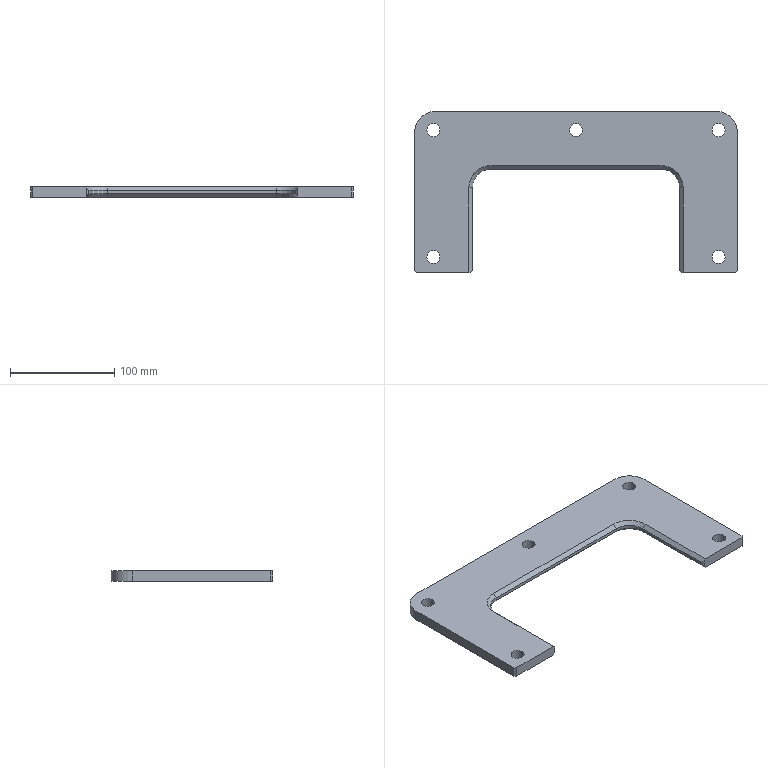Part | SolidWorks | features Chamfer 2, Extrusion 1, ICE 1 | 1 solid | 38 faces | box 310 x 155 x 10 mm | volume 271244 mm3 | plane 20 | cylinder 14 | cone 4 | commonest cylinder face diameters 12.5 x10 36 x2 40 x2
STEP:
#1=CARTESIAN_POINT('',(-143.25,15.,0.));
#2=VERTEX_POINT('',#1);
#3=CARTESIAN_POINT('',(-130.75,15.,0.));
#4=VERTEX_POINT('',#3);
#5=CARTESIAN_POINT('',(-137.,15.,0.));
#6=DIRECTION('',(0.,0.,1.));
#7=DIRECTION('',(1.,0.,0.));
#8=AXIS2_PLACEMENT_3D('',#5,#6,#7);
#9=CIRCLE('',#8,6.25);
#10=EDGE_CURVE('',#2,#4,#9,.T.);
#11=ORIENTED_EDGE('',*,*,#10,.F.);
#12=CARTESIAN_POINT('',(-143.25,15.,10.));
#13=VERTEX_POINT('',#12);
#14=CARTESIAN_POINT('',(-143.25,15.,0.));
#15=DIRECTION('',(0.,0.,1.));
#16=VECTOR('',#15,1000.);
#17=LINE('',#14,#16);
#18=EDGE_CURVE('',#2,#13,#17,.T.);
#19=ORIENTED_EDGE('',*,*,#18,.T.);
#20=CARTESIAN_POINT('',(-130.75,15.,10.));
#21=VERTEX_POINT('',#20);
#22=CARTESIAN_POINT('',(-137.,15.,10.));
#23=DIRECTION('',(0.,0.,1.));
#24=DIRECTION('',(1.,0.,0.));
#25=AXIS2_PLACEMENT_3D('',#22,#23,#24);
#26=CIRCLE('',#25,6.25);
#27=EDGE_CURVE('',#13,#21,#26,.T.);
#28=ORIENTED_EDGE('',*,*,#27,.T.);
#29=CARTESIAN_POINT('',(-130.75,15.,0.));
#30=DIRECTION('',(0.,0.,1.));
#31=VECTOR('',#30,1000.);
#32=LINE('',#29,#31);
#33=EDGE_CURVE('',#4,#21,#32,.T.);
#34=ORIENTED_EDGE('',*,*,#33,.F.);
#35=EDGE_LOOP('',(#11,#19,#28,#34));
#36=FACE_OUTER_BOUND('',#35,.T.);
#37=CARTESIAN_POINT('',(-137.,15.,0.));
#38=DIRECTION('',(0.,0.,1.));
#39=DIRECTION('',(1.,0.,0.));
#40=AXIS2_PLACEMENT_3D('',#37,#38,#39);
#41=CYLINDRICAL_SURFACE('',#40,6.25);
#42=ADVANCED_FACE('',(#36),#41,.F.);
#43=CARTESIAN_POINT('',(130.75,15.,0.));
#44=VERTEX_POINT('',#43);
#45=CARTESIAN_POINT('',(143.25,15.,0.));
#46=VERTEX_POINT('',#45);
#47=CARTESIAN_POINT('',(137.,15.,0.));
#48=DIRECTION('',(0.,0.,1.));
#49=DIRECTION('',(-1.,0.,0.));
#50=AXIS2_PLACEMENT_3D('',#47,#48,#49);
#51=CIRCLE('',#50,6.25);
#52=EDGE_CURVE('',#44,#46,#51,.T.);
#53=ORIENTED_EDGE('',*,*,#52,.F.);
#54=CARTESIAN_POINT('',(130.75,15.,10.));
#55=VERTEX_POINT('',#54);
#56=CARTESIAN_POINT('',(130.75,15.,0.));
#57=DIRECTION('',(0.,0.,1.));
#58=VECTOR('',#57,1000.);
#59=LINE('',#56,#58);
#60=EDGE_CURVE('',#44,#55,#59,.T.);
#61=ORIENTED_EDGE('',*,*,#60,.T.);
#62=CARTESIAN_POINT('',(143.25,15.,10.));
#63=VERTEX_POINT('',#62);
#64=CARTESIAN_POINT('',(137.,15.,10.));
#65=DIRECTION('',(0.,0.,1.));
#66=DIRECTION('',(-1.,0.,0.));
#67=AXIS2_PLACEMENT_3D('',#64,#65,#66);
#68=CIRCLE('',#67,6.25);
#69=EDGE_CURVE('',#55,#63,#68,.T.);
#70=ORIENTED_EDGE('',*,*,#69,.T.);
#71=CARTESIAN_POINT('',(143.25,15.,0.));
#72=DIRECTION('',(0.,0.,1.));
#73=VECTOR('',#72,1000.);
#74=LINE('',#71,#73);
#75=EDGE_CURVE('',#46,#63,#74,.T.);
#76=ORIENTED_EDGE('',*,*,#75,.F.);
#77=EDGE_LOOP('',(#53,#61,#70,#76));
#78=FACE_OUTER_BOUND('',#77,.T.);
#79=CARTESIAN_POINT('',(137.,15.,0.));
#80=DIRECTION('',(0.,0.,1.));
#81=DIRECTION('',(1.,0.,0.));
#82=AXIS2_PLACEMENT_3D('',#79,#80,#81);
#83=CYLINDRICAL_SURFACE('',#82,6.25);
#84=ADVANCED_FACE('',(#78),#83,.F.);
#85=CARTESIAN_POINT('',(-143.25,137.,0.));
#86=VERTEX_POINT('',#85);
#87=CARTESIAN_POINT('',(-130.75,137.,0.));
#88=VERTEX_POINT('',#87);
#89=CARTESIAN_POINT('',(-137.,137.,0.));
#90=DIRECTION('',(0.,0.,1.));
#91=DIRECTION('',(1.,0.,0.));
#92=AXIS2_PLACEMENT_3D('',#89,#90,#91);
#93=CIRCLE('',#92,6.25);
#94=EDGE_CURVE('',#86,#88,#93,.T.);
#95=ORIENTED_EDGE('',*,*,#94,.F.);
#96=CARTESIAN_POINT('',(-143.25,137.,10.));
#97=VERTEX_POINT('',#96);
#98=CARTESIAN_POINT('',(-143.25,137.,0.));
#99=DIRECTION('',(0.,0.,1.));
#100=VECTOR('',#99,1000.);
#101=LINE('',#98,#100);
#102=EDGE_CURVE('',#86,#97,#101,.T.);
#103=ORIENTED_EDGE('',*,*,#102,.T.);
#104=CARTESIAN_POINT('',(-130.75,137.,10.));
#105=VERTEX_POINT('',#104);
#106=CARTESIAN_POINT('',(-137.,137.,10.));
#107=DIRECTION('',(0.,0.,1.));
#108=DIRECTION('',(1.,0.,0.));
#109=AXIS2_PLACEMENT_3D('',#106,#107,#108);
#110=CIRCLE('',#109,6.25);
#111=EDGE_CURVE('',#97,#105,#110,.T.);
#112=ORIENTED_EDGE('',*,*,#111,.T.);
#113=CARTESIAN_POINT('',(-130.75,137.,0.));
#114=DIRECTION('',(0.,0.,1.));
#115=VECTOR('',#114,1000.);
#116=LINE('',#113,#115);
#117=EDGE_CURVE('',#88,#105,#116,.T.);
#118=ORIENTED_EDGE('',*,*,#117,.F.);
#119=EDGE_LOOP('',(#95,#103,#112,#118));
#120=FACE_OUTER_BOUND('',#119,.T.);
#121=CARTESIAN_POINT('',(-137.,137.,0.));
#122=DIRECTION('',(0.,0.,1.));
#123=DIRECTION('',(1.,0.,0.));
#124=AXIS2_PLACEMENT_3D('',#121,#122,#123);
#125=CYLINDRICAL_SURFACE('',#124,6.25);
#126=ADVANCED_FACE('',(#120),#125,.F.);
#127=CARTESIAN_POINT('',(130.75,137.,0.));
#128=VERTEX_POINT('',#127);
#129=CARTESIAN_POINT('',(143.25,137.,0.));
#130=VERTEX_POINT('',#129);
#131=CARTESIAN_POINT('',(137.,137.,0.));
#132=DIRECTION('',(0.,0.,1.));
#133=DIRECTION('',(1.,0.,0.));
#134=AXIS2_PLACEMENT_3D('',#131,#132,#133);
#135=CIRCLE('',#134,6.25);
#136=EDGE_CURVE('',#128,#130,#135,.T.);
#137=ORIENTED_EDGE('',*,*,#136,.F.);
#138=CARTESIAN_POINT('',(130.75,137.,10.));
#139=VERTEX_POINT('',#138);
#140=CARTESIAN_POINT('',(130.75,137.,0.));
#141=DIRECTION('',(0.,0.,1.));
#142=VECTOR('',#141,1000.);
#143=LINE('',#140,#142);
#144=EDGE_CURVE('',#128,#139,#143,.T.);
#145=ORIENTED_EDGE('',*,*,#144,.T.);
#146=CARTESIAN_POINT('',(143.25,137.,10.));
#147=VERTEX_POINT('',#146);
#148=CARTESIAN_POINT('',(137.,137.,10.));
#149=DIRECTION('',(0.,0.,1.));
#150=DIRECTION('',(1.,0.,0.));
#151=AXIS2_PLACEMENT_3D('',#148,#149,#150);
#152=CIRCLE('',#151,6.25);
#153=EDGE_CURVE('',#139,#147,#152,.T.);
#154=ORIENTED_EDGE('',*,*,#153,.T.);
#155=CARTESIAN_POINT('',(143.25,137.,0.));
#156=DIRECTION('',(0.,0.,1.));
#157=VECTOR('',#156,1000.);
#158=LINE('',#155,#157);
#159=EDGE_CURVE('',#130,#147,#158,.T.);
#160=ORIENTED_EDGE('',*,*,#159,.F.);
#161=EDGE_LOOP('',(#137,#145,#154,#160));
#162=FACE_OUTER_BOUND('',#161,.T.);
#163=CARTESIAN_POINT('',(137.,137.,0.));
#164=DIRECTION('',(0.,0.,1.));
#165=DIRECTION('',(1.,0.,0.));
#166=AXIS2_PLACEMENT_3D('',#163,#164,#165);
#167=CYLINDRICAL_SURFACE('',#166,6.25);
#168=ADVANCED_FACE('',(#162),#167,.F.);
#169=CARTESIAN_POINT('',(-6.25,137.,0.));
#170=VERTEX_POINT('',#169);
#171=CARTESIAN_POINT('',(6.25,137.,0.));
#172=VERTEX_POINT('',#171);
#173=CARTESIAN_POINT('',(0.,137.,0.));
#174=DIRECTION('',(0.,0.,1.));
#175=DIRECTION('',(1.,0.,0.));
#176=AXIS2_PLACEMENT_3D('',#173,#174,#175);
#177=CIRCLE('',#176,6.25);
#178=EDGE_CURVE('',#170,#172,#177,.T.);
#179=ORIENTED_EDGE('',*,*,#178,.F.);
#180=CARTESIAN_POINT('',(-6.25,137.,10.));
#181=VERTEX_POINT('',#180);
#182=CARTESIAN_POINT('',(-6.25,137.,0.));
#183=DIRECTION('',(0.,0.,1.));
#184=VECTOR('',#183,1000.);
#185=LINE('',#182,#184);
#186=EDGE_CURVE('',#170,#181,#185,.T.);
#187=ORIENTED_EDGE('',*,*,#186,.T.);
#188=CARTESIAN_POINT('',(6.25,137.,10.));
#189=VERTEX_POINT('',#188);
#190=CARTESIAN_POINT('',(0.,137.,10.));
#191=DIRECTION('',(0.,0.,1.));
#192=DIRECTION('',(1.,0.,0.));
#193=AXIS2_PLACEMENT_3D('',#190,#191,#192);
#194=CIRCLE('',#193,6.25);
#195=EDGE_CURVE('',#181,#189,#194,.T.);
#196=ORIENTED_EDGE('',*,*,#195,.T.);
#197=CARTESIAN_POINT('',(6.25,137.,0.));
#198=DIRECTION('',(0.,0.,1.));
#199=VECTOR('',#198,1000.);
#200=LINE('',#197,#199);
#201=EDGE_CURVE('',#172,#189,#200,.T.);
#202=ORIENTED_EDGE('',*,*,#201,.F.);
#203=EDGE_LOOP('',(#179,#187,#196,#202));
#204=FACE_OUTER_BOUND('',#203,.T.);
#205=CARTESIAN_POINT('',(0.,137.,0.));
#206=DIRECTION('',(0.,0.,1.));
#207=DIRECTION('',(1.,0.,0.));
#208=AXIS2_PLACEMENT_3D('',#205,#206,#207);
#209=CYLINDRICAL_SURFACE('',#208,6.25);
#210=ADVANCED_FACE('',(#204),#209,.F.);
#211=CARTESIAN_POINT('',(81.5,99.5,6.5));
#212=VERTEX_POINT('',#211);
#213=CARTESIAN_POINT('',(81.5,99.5,3.5));
#214=VERTEX_POINT('',#213);
#215=CARTESIAN_POINT('',(81.5,99.5,10.));
#216=DIRECTION('',(0.,0.,-1.));
#217=VECTOR('',#216,1000.);
#218=LINE('',#215,#217);
#219=EDGE_CURVE('',#212,#214,#218,.T.);
#220=ORIENTED_EDGE('',*,*,#219,.T.);
#221=CARTESIAN_POINT('',(99.5,81.5,3.5));
#222=VERTEX_POINT('',#221);
#223=CARTESIAN_POINT('',(81.5,81.5,3.5));
#224=DIRECTION('',(0.,0.,-1.));
#225=DIRECTION('',(1.,0.,0.));
#226=AXIS2_PLACEMENT_3D('',#223,#224,#225);
#227=CIRCLE('',#226,18.);
#228=EDGE_CURVE('',#214,#222,#227,.T.);
#229=ORIENTED_EDGE('',*,*,#228,.T.);
#230=CARTESIAN_POINT('',(99.5,81.5,6.5));
#231=VERTEX_POINT('',#230);
#232=CARTESIAN_POINT('',(99.5,81.5,10.));
#233=DIRECTION('',(0.,0.,-1.));
#234=VECTOR('',#233,1000.);
#235=LINE('',#232,#234);
#236=EDGE_CURVE('',#231,#222,#235,.T.);
#237=ORIENTED_EDGE('',*,*,#236,.F.);
#238=CARTESIAN_POINT('',(81.5,81.5,6.5));
#239=DIRECTION('',(0.,0.,1.));
#240=DIRECTION('',(1.,0.,0.));
#241=AXIS2_PLACEMENT_3D('',#238,#239,#240);
#242=CIRCLE('',#241,18.);
#243=EDGE_CURVE('',#231,#212,#242,.T.);
#244=ORIENTED_EDGE('',*,*,#243,.T.);
#245=EDGE_LOOP('',(#220,#229,#237,#244));
#246=FACE_OUTER_BOUND('',#245,.T.);
#247=CARTESIAN_POINT('',(81.5,81.5,10.));
#248=DIRECTION('',(0.,0.,-1.));
#249=DIRECTION('',(-1.,0.,0.));
#250=AXIS2_PLACEMENT_3D('',#247,#248,#249);
#251=CYLINDRICAL_SURFACE('',#250,18.);
#252=ADVANCED_FACE('',(#246),#251,.F.);
#253=ORIENTED_EDGE('',*,*,#236,.T.);
#254=CARTESIAN_POINT('',(99.5,2.,3.5));
#255=VERTEX_POINT('',#254);
#256=CARTESIAN_POINT('',(99.5,2.5,3.5));
#257=DIRECTION('',(0.,-1.,0.));
#258=VECTOR('',#257,1000.);
#259=LINE('',#256,#258);
#260=EDGE_CURVE('',#222,#255,#259,.T.);
#261=ORIENTED_EDGE('',*,*,#260,.T.);
#262=CARTESIAN_POINT('',(99.5,2.,6.5));
#263=VERTEX_POINT('',#262);
#264=CARTESIAN_POINT('',(99.5,2.,10.));
#265=DIRECTION('',(0.,0.,1.));
#266=VECTOR('',#265,1000.);
#267=LINE('',#264,#266);
#268=EDGE_CURVE('',#255,#263,#267,.T.);
#269=ORIENTED_EDGE('',*,*,#268,.T.);
#270=CARTESIAN_POINT('',(99.5,81.5,6.5));
#271=DIRECTION('',(0.,1.,0.));
#272=VECTOR('',#271,1000.);
#273=LINE('',#270,#272);
#274=EDGE_CURVE('',#263,#231,#273,.T.);
#275=ORIENTED_EDGE('',*,*,#274,.T.);
#276=EDGE_LOOP('',(#253,#261,#269,#275));
#277=FACE_OUTER_BOUND('',#276,.T.);
#278=CARTESIAN_POINT('',(99.5,2.5,10.));
#279=DIRECTION('',(1.,0.,0.));
#280=DIRECTION('',(0.,1.,0.));
#281=AXIS2_PLACEMENT_3D('',#278,#279,#280);
#282=PLANE('',#281);
#283=ADVANCED_FACE('',(#277),#282,.F.);
#284=CARTESIAN_POINT('',(101.5,0.,8.5));
#285=VERTEX_POINT('',#284);
#286=CARTESIAN_POINT('',(101.5,0.,1.5));
#287=VERTEX_POINT('',#286);
#288=CARTESIAN_POINT('',(101.5,0.,10.));
#289=DIRECTION('',(0.,0.,-1.));
#290=VECTOR('',#289,1000.);
#291=LINE('',#288,#290);
#292=EDGE_CURVE('',#285,#287,#291,.T.);
#293=ORIENTED_EDGE('',*,*,#292,.T.);
#294=CARTESIAN_POINT('',(103.,0.,0.));
#295=VERTEX_POINT('',#294);
#296=CARTESIAN_POINT('',(99.5,0.,3.5));
#297=DIRECTION('',(0.7071,0.,-0.7071));
#298=VECTOR('',#297,1000.);
#299=LINE('',#296,#298);
#300=EDGE_CURVE('',#287,#295,#299,.T.);
#301=ORIENTED_EDGE('',*,*,#300,.T.);
#302=CARTESIAN_POINT('',(153.,0.,0.));
#303=VERTEX_POINT('',#302);
#304=CARTESIAN_POINT('',(99.5,0.,0.));
#305=DIRECTION('',(1.,0.,0.));
#306=VECTOR('',#305,1000.);
#307=LINE('',#304,#306);
#308=EDGE_CURVE('',#295,#303,#307,.T.);
#309=ORIENTED_EDGE('',*,*,#308,.T.);
#310=CARTESIAN_POINT('',(153.,0.,10.));
#311=VERTEX_POINT('',#310);
#312=CARTESIAN_POINT('',(153.,0.,10.));
#313=DIRECTION('',(0.,0.,1.));
#314=VECTOR('',#313,1000.);
#315=LINE('',#312,#314);
#316=EDGE_CURVE('',#303,#311,#315,.T.);
#317=ORIENTED_EDGE('',*,*,#316,.T.);
#318=CARTESIAN_POINT('',(103.,0.,10.));
#319=VERTEX_POINT('',#318);
#320=CARTESIAN_POINT('',(99.5,0.,10.));
#321=DIRECTION('',(1.,0.,0.));
#322=VECTOR('',#321,1000.);
#323=LINE('',#320,#322);
#324=EDGE_CURVE('',#319,#311,#323,.T.);
#325=ORIENTED_EDGE('',*,*,#324,.F.);
#326=CARTESIAN_POINT('',(103.,0.,10.));
#327=DIRECTION('',(-0.7071,0.,-0.7071));
#328=VECTOR('',#327,1000.);
#329=LINE('',#326,#328);
#330=EDGE_CURVE('',#319,#285,#329,.T.);
#331=ORIENTED_EDGE('',*,*,#330,.T.);
#332=EDGE_LOOP('',(#293,#301,#309,#317,#325,#331));
#333=FACE_OUTER_BOUND('',#332,.T.);
#334=CARTESIAN_POINT('',(99.5,0.,10.));
#335=DIRECTION('',(0.,1.,0.));
#336=DIRECTION('',(-1.,0.,0.));
#337=AXIS2_PLACEMENT_3D('',#334,#335,#336);
#338=PLANE('',#337);
#339=ADVANCED_FACE('',(#333),#338,.F.);
#340=CARTESIAN_POINT('',(155.,2.,10.));
#341=VERTEX_POINT('',#340);
#342=CARTESIAN_POINT('',(155.,135.,10.));
#343=VERTEX_POINT('',#342);
#344=CARTESIAN_POINT('',(155.,2.5,10.));
#345=DIRECTION('',(0.,1.,0.));
#346=VECTOR('',#345,1000.);
#347=LINE('',#344,#346);
#348=EDGE_CURVE('',#341,#343,#347,.T.);
#349=ORIENTED_EDGE('',*,*,#348,.F.);
#350=CARTESIAN_POINT('',(155.,2.,0.));
#351=VERTEX_POINT('',#350);
#352=CARTESIAN_POINT('',(155.,2.,10.));
#353=DIRECTION('',(0.,0.,-1.));
#354=VECTOR('',#353,1000.);
#355=LINE('',#352,#354);
#356=EDGE_CURVE('',#341,#351,#355,.T.);
#357=ORIENTED_EDGE('',*,*,#356,.T.);
#358=CARTESIAN_POINT('',(155.,135.,0.));
#359=VERTEX_POINT('',#358);
#360=CARTESIAN_POINT('',(155.,2.5,0.));
#361=DIRECTION('',(0.,1.,0.));
#362=VECTOR('',#361,1000.);
#363=LINE('',#360,#362);
#364=EDGE_CURVE('',#351,#359,#363,.T.);
#365=ORIENTED_EDGE('',*,*,#364,.T.);
#366=CARTESIAN_POINT('',(155.,135.,10.));
#367=DIRECTION('',(0.,0.,-1.));
#368=VECTOR('',#367,1000.);
#369=LINE('',#366,#368);
#370=EDGE_CURVE('',#343,#359,#369,.T.);
#371=ORIENTED_EDGE('',*,*,#370,.F.);
#372=EDGE_LOOP('',(#349,#357,#365,#371));
#373=FACE_OUTER_BOUND('',#372,.T.);
#374=CARTESIAN_POINT('',(155.,2.5,10.));
#375=DIRECTION('',(-1.,0.,0.));
#376=DIRECTION('',(0.,0.,1.));
#377=AXIS2_PLACEMENT_3D('',#374,#375,#376);
#378=PLANE('',#377);
#379=ADVANCED_FACE('',(#373),#378,.F.);
#380=CARTESIAN_POINT('',(135.,155.,0.));
#381=VERTEX_POINT('',#380);
#382=CARTESIAN_POINT('',(135.,135.,0.));
#383=DIRECTION('',(0.,0.,1.));
#384=DIRECTION('',(1.,0.,0.));
#385=AXIS2_PLACEMENT_3D('',#382,#383,#384);
#386=CIRCLE('',#385,20.);
#387=EDGE_CURVE('',#359,#381,#386,.T.);
#388=ORIENTED_EDGE('',*,*,#387,.T.);
#389=CARTESIAN_POINT('',(135.,155.,10.));
#390=VERTEX_POINT('',#389);
#391=CARTESIAN_POINT('',(135.,155.,10.));
#392=DIRECTION('',(0.,0.,-1.));
#393=VECTOR('',#392,1000.);
#394=LINE('',#391,#393);
#395=EDGE_CURVE('',#390,#381,#394,.T.);
#396=ORIENTED_EDGE('',*,*,#395,.F.);
#397=CARTESIAN_POINT('',(135.,135.,10.));
#398=DIRECTION('',(0.,0.,1.));
#399=DIRECTION('',(1.,0.,0.));
#400=AXIS2_PLACEMENT_3D('',#397,#398,#399);
#401=CIRCLE('',#400,20.);
#402=EDGE_CURVE('',#343,#390,#401,.T.);
#403=ORIENTED_EDGE('',*,*,#402,.F.);
#404=ORIENTED_EDGE('',*,*,#370,.T.);
#405=EDGE_LOOP('',(#388,#396,#403,#404));
#406=FACE_OUTER_BOUND('',#405,.T.);
#407=CARTESIAN_POINT('',(135.,135.,10.));
#408=DIRECTION('',(0.,0.,-1.));
#409=DIRECTION('',(-1.,0.,0.));
#410=AXIS2_PLACEMENT_3D('',#407,#408,#409);
#411=CYLINDRICAL_SURFACE('',#410,20.);
#412=ADVANCED_FACE('',(#406),#411,.T.);
#413=CARTESIAN_POINT('',(-135.,155.,0.));
#414=VERTEX_POINT('',#413);
#415=CARTESIAN_POINT('',(-135.,155.,0.));
#416=DIRECTION('',(-1.,0.,0.));
#417=VECTOR('',#416,1000.);
#418=LINE('',#415,#417);
#419=EDGE_CURVE('',#381,#414,#418,.T.);
#420=ORIENTED_EDGE('',*,*,#419,.T.);
#421=CARTESIAN_POINT('',(-135.,155.,10.));
#422=VERTEX_POINT('',#421);
#423=CARTESIAN_POINT('',(-135.,155.,10.));
#424=DIRECTION('',(0.,0.,-1.));
#425=VECTOR('',#424,1000.);
#426=LINE('',#423,#425);
#427=EDGE_CURVE('',#422,#414,#426,.T.);
#428=ORIENTED_EDGE('',*,*,#427,.F.);
#429=CARTESIAN_POINT('',(-135.,155.,10.));
#430=DIRECTION('',(-1.,0.,0.));
#431=VECTOR('',#430,1000.);
#432=LINE('',#429,#431);
#433=EDGE_CURVE('',#390,#422,#432,.T.);
#434=ORIENTED_EDGE('',*,*,#433,.F.);
#435=ORIENTED_EDGE('',*,*,#395,.T.);
#436=EDGE_LOOP('',(#420,#428,#434,#435));
#437=FACE_OUTER_BOUND('',#436,.T.);
#438=CARTESIAN_POINT('',(-135.,155.,10.));
#439=DIRECTION('',(0.,-1.,0.));
#440=DIRECTION('',(0.,0.,-1.));
#441=AXIS2_PLACEMENT_3D('',#438,#439,#440);
#442=PLANE('',#441);
#443=ADVANCED_FACE('',(#437),#442,.F.);
#444=CARTESIAN_POINT('',(-155.,135.,0.));
#445=VERTEX_POINT('',#444);
#446=CARTESIAN_POINT('',(-135.,135.,0.));
#447=DIRECTION('',(0.,0.,1.));
#448=DIRECTION('',(-1.,0.,0.));
#449=AXIS2_PLACEMENT_3D('',#446,#447,#448);
#450=CIRCLE('',#449,20.);
#451=EDGE_CURVE('',#414,#445,#450,.T.);
#452=ORIENTED_EDGE('',*,*,#451,.T.);
#453=CARTESIAN_POINT('',(-155.,135.,10.));
#454=VERTEX_POINT('',#453);
#455=CARTESIAN_POINT('',(-155.,135.,10.));
#456=DIRECTION('',(0.,0.,-1.));
#457=VECTOR('',#456,1000.);
#458=LINE('',#455,#457);
#459=EDGE_CURVE('',#454,#445,#458,.T.);
#460=ORIENTED_EDGE('',*,*,#459,.F.);
#461=CARTESIAN_POINT('',(-135.,135.,10.));
#462=DIRECTION('',(0.,0.,1.));
#463=DIRECTION('',(-1.,0.,0.));
#464=AXIS2_PLACEMENT_3D('',#461,#462,#463);
#465=CIRCLE('',#464,20.);
#466=EDGE_CURVE('',#422,#454,#465,.T.);
#467=ORIENTED_EDGE('',*,*,#466,.F.);
#468=ORIENTED_EDGE('',*,*,#427,.T.);
#469=EDGE_LOOP('',(#452,#460,#467,#468));
#470=FACE_OUTER_BOUND('',#469,.T.);
#471=CARTESIAN_POINT('',(-135.,135.,10.));
#472=DIRECTION('',(0.,0.,-1.));
#473=DIRECTION('',(-1.,0.,0.));
#474=AXIS2_PLACEMENT_3D('',#471,#472,#473);
#475=CYLINDRICAL_SURFACE('',#474,20.);
#476=ADVANCED_FACE('',(#470),#475,.T.);
#477=CARTESIAN_POINT('',(-155.,2.,0.));
#478=VERTEX_POINT('',#477);
#479=CARTESIAN_POINT('',(-155.,2.5,0.));
#480=DIRECTION('',(0.,-1.,0.));
#481=VECTOR('',#480,1000.);
#482=LINE('',#479,#481);
#483=EDGE_CURVE('',#445,#478,#482,.T.);
#484=ORIENTED_EDGE('',*,*,#483,.T.);
#485=CARTESIAN_POINT('',(-155.,2.,10.));
#486=VERTEX_POINT('',#485);
#487=CARTESIAN_POINT('',(-155.,2.,10.));
#488=DIRECTION('',(0.,0.,1.));
#489=VECTOR('',#488,1000.);
#490=LINE('',#487,#489);
#491=EDGE_CURVE('',#478,#486,#490,.T.);
#492=ORIENTED_EDGE('',*,*,#491,.T.);
#493=CARTESIAN_POINT('',(-155.,2.5,10.));
#494=DIRECTION('',(0.,-1.,0.));
#495=VECTOR('',#494,1000.);
#496=LINE('',#493,#495);
#497=EDGE_CURVE('',#454,#486,#496,.T.);
#498=ORIENTED_EDGE('',*,*,#497,.F.);
#499=ORIENTED_EDGE('',*,*,#459,.T.);
#500=EDGE_LOOP('',(#484,#492,#498,#499));
#501=FACE_OUTER_BOUND('',#500,.T.);
#502=CARTESIAN_POINT('',(-155.,2.5,10.));
#503=DIRECTION('',(1.,0.,0.));
#504=DIRECTION('',(0.,0.,-1.));
#505=AXIS2_PLACEMENT_3D('',#502,#503,#504);
#506=PLANE('',#505);
#507=ADVANCED_FACE('',(#501),#506,.F.);
#508=CARTESIAN_POINT('',(-153.,0.,0.));
#509=VERTEX_POINT('',#508);
#510=CARTESIAN_POINT('',(-103.,0.,0.));
#511=VERTEX_POINT('',#510);
#512=CARTESIAN_POINT('',(-155.,0.,0.));
#513=DIRECTION('',(1.,0.,0.));
#514=VECTOR('',#513,1000.);
#515=LINE('',#512,#514);
#516=EDGE_CURVE('',#509,#511,#515,.T.);
#517=ORIENTED_EDGE('',*,*,#516,.T.);
#518=CARTESIAN_POINT('',(-101.5,0.,1.5));
#519=VERTEX_POINT('',#518);
#520=CARTESIAN_POINT('',(-99.5,0.,3.5));
#521=DIRECTION('',(0.7071,0.,0.7071));
#522=VECTOR('',#521,1000.);
#523=LINE('',#520,#522);
#524=EDGE_CURVE('',#511,#519,#523,.T.);
#525=ORIENTED_EDGE('',*,*,#524,.T.);
#526=CARTESIAN_POINT('',(-101.5,0.,8.5));
#527=VERTEX_POINT('',#526);
#528=CARTESIAN_POINT('',(-101.5,0.,10.));
#529=DIRECTION('',(0.,0.,1.));
#530=VECTOR('',#529,1000.);
#531=LINE('',#528,#530);
#532=EDGE_CURVE('',#519,#527,#531,.T.);
#533=ORIENTED_EDGE('',*,*,#532,.T.);
#534=CARTESIAN_POINT('',(-103.,0.,10.));
#535=VERTEX_POINT('',#534);
#536=CARTESIAN_POINT('',(-103.,0.,10.));
#537=DIRECTION('',(-0.7071,0.,0.7071));
#538=VECTOR('',#537,1000.);
#539=LINE('',#536,#538);
#540=EDGE_CURVE('',#527,#535,#539,.T.);
#541=ORIENTED_EDGE('',*,*,#540,.T.);
#542=CARTESIAN_POINT('',(-153.,0.,10.));
#543=VERTEX_POINT('',#542);
#544=CARTESIAN_POINT('',(-155.,0.,10.));
#545=DIRECTION('',(1.,0.,0.));
#546=VECTOR('',#545,1000.);
#547=LINE('',#544,#546);
#548=EDGE_CURVE('',#543,#535,#547,.T.);
#549=ORIENTED_EDGE('',*,*,#548,.F.);
#550=CARTESIAN_POINT('',(-153.,0.,10.));
#551=DIRECTION('',(0.,0.,-1.));
#552=VECTOR('',#551,1000.);
#553=LINE('',#550,#552);
#554=EDGE_CURVE('',#543,#509,#553,.T.);
#555=ORIENTED_EDGE('',*,*,#554,.T.);
#556=EDGE_LOOP('',(#517,#525,#533,#541,#549,#555));
#557=FACE_OUTER_BOUND('',#556,.T.);
#558=CARTESIAN_POINT('',(-155.,0.,10.));
#559=DIRECTION('',(0.,1.,0.));
#560=DIRECTION('',(-1.,0.,0.));
#561=AXIS2_PLACEMENT_3D('',#558,#559,#560);
#562=PLANE('',#561);
#563=ADVANCED_FACE('',(#557),#562,.F.);
#564=CARTESIAN_POINT('',(-99.5,2.,6.5));
#565=VERTEX_POINT('',#564);
#566=CARTESIAN_POINT('',(-99.5,2.,3.5));
#567=VERTEX_POINT('',#566);
#568=CARTESIAN_POINT('',(-99.5,2.,10.));
#569=DIRECTION('',(0.,0.,-1.));
#570=VECTOR('',#569,1000.);
#571=LINE('',#568,#570);
#572=EDGE_CURVE('',#565,#567,#571,.T.);
#573=ORIENTED_EDGE('',*,*,#572,.T.);
#574=CARTESIAN_POINT('',(-99.5,81.5,3.5));
#575=VERTEX_POINT('',#574);
#576=CARTESIAN_POINT('',(-99.5,81.5,3.5));
#577=DIRECTION('',(0.,1.,0.));
#578=VECTOR('',#577,1000.);
#579=LINE('',#576,#578);
#580=EDGE_CURVE('',#567,#575,#579,.T.);
#581=ORIENTED_EDGE('',*,*,#580,.T.);
#582=CARTESIAN_POINT('',(-99.5,81.5,6.5));
#583=VERTEX_POINT('',#582);
#584=CARTESIAN_POINT('',(-99.5,81.5,10.));
#585=DIRECTION('',(0.,0.,-1.));
#586=VECTOR('',#585,1000.);
#587=LINE('',#584,#586);
#588=EDGE_CURVE('',#583,#575,#587,.T.);
#589=ORIENTED_EDGE('',*,*,#588,.F.);
#590=CARTESIAN_POINT('',(-99.5,2.,6.5));
#591=DIRECTION('',(0.,-1.,0.));
#592=VECTOR('',#591,1000.);
#593=LINE('',#590,#592);
#594=EDGE_CURVE('',#583,#565,#593,.T.);
#595=ORIENTED_EDGE('',*,*,#594,.T.);
#596=EDGE_LOOP('',(#573,#581,#589,#595));
#597=FACE_OUTER_BOUND('',#596,.T.);
#598=CARTESIAN_POINT('',(-99.5,81.5,10.));
#599=DIRECTION('',(-1.,0.,0.));
#600=DIRECTION('',(0.,-1.,0.));
#601=AXIS2_PLACEMENT_3D('',#598,#599,#600);
#602=PLANE('',#601);
#603=ADVANCED_FACE('',(#597),#602,.F.);
#604=ORIENTED_EDGE('',*,*,#588,.T.);
#605=CARTESIAN_POINT('',(-81.5,99.5,3.5));
#606=VERTEX_POINT('',#605);
#607=CARTESIAN_POINT('',(-81.5,81.5,3.5));
#608=DIRECTION('',(0.,0.,-1.));
#609=DIRECTION('',(1.,0.,0.));
#610=AXIS2_PLACEMENT_3D('',#607,#608,#609);
#611=CIRCLE('',#610,18.);
#612=EDGE_CURVE('',#575,#606,#611,.T.);
#613=ORIENTED_EDGE('',*,*,#612,.T.);
#614=CARTESIAN_POINT('',(-81.5,99.5,6.5));
#615=VERTEX_POINT('',#614);
#616=CARTESIAN_POINT('',(-81.5,99.5,10.));
#617=DIRECTION('',(0.,0.,-1.));
#618=VECTOR('',#617,1000.);
#619=LINE('',#616,#618);
#620=EDGE_CURVE('',#615,#606,#619,.T.);
#621=ORIENTED_EDGE('',*,*,#620,.F.);
#622=CARTESIAN_POINT('',(-81.5,81.5,6.5));
#623=DIRECTION('',(0.,0.,1.));
#624=DIRECTION('',(1.,0.,0.));
#625=AXIS2_PLACEMENT_3D('',#622,#623,#624);
#626=CIRCLE('',#625,18.);
#627=EDGE_CURVE('',#615,#583,#626,.T.);
#628=ORIENTED_EDGE('',*,*,#627,.T.);
#629=EDGE_LOOP('',(#604,#613,#621,#628));
#630=FACE_OUTER_BOUND('',#629,.T.);
#631=CARTESIAN_POINT('',(-81.5,81.5,10.));
#632=DIRECTION('',(0.,0.,-1.));
#633=DIRECTION('',(-1.,0.,0.));
#634=AXIS2_PLACEMENT_3D('',#631,#632,#633);
#635=CYLINDRICAL_SURFACE('',#634,18.);
#636=ADVANCED_FACE('',(#630),#635,.F.);
#637=ORIENTED_EDGE('',*,*,#620,.T.);
#638=CARTESIAN_POINT('',(-81.5,99.5,3.5));
#639=DIRECTION('',(1.,0.,0.));
#640=VECTOR('',#639,1000.);
#641=LINE('',#638,#640);
#642=EDGE_CURVE('',#606,#214,#641,.T.);
#643=ORIENTED_EDGE('',*,*,#642,.T.);
#644=ORIENTED_EDGE('',*,*,#219,.F.);
#645=CARTESIAN_POINT('',(-81.5,99.5,6.5));
#646=DIRECTION('',(-1.,0.,0.));
#647=VECTOR('',#646,1000.);
#648=LINE('',#645,#647);
#649=EDGE_CURVE('',#212,#615,#648,.T.);
#650=ORIENTED_EDGE('',*,*,#649,.T.);
#651=EDGE_LOOP('',(#637,#643,#644,#650));
#652=FACE_OUTER_BOUND('',#651,.T.);
#653=CARTESIAN_POINT('',(-81.5,99.5,10.));
#654=DIRECTION('',(0.,1.,0.));
#655=DIRECTION('',(0.,0.,1.));
#656=AXIS2_PLACEMENT_3D('',#653,#654,#655);
#657=PLANE('',#656);
#658=ADVANCED_FACE('',(#652),#657,.F.);
#659=CARTESIAN_POINT('',(-137.,15.,10.));
#660=DIRECTION('',(0.,0.,1.));
#661=DIRECTION('',(1.,0.,0.));
#662=AXIS2_PLACEMENT_3D('',#659,#660,#661);
#663=CIRCLE('',#662,6.25);
#664=EDGE_CURVE('',#21,#13,#663,.T.);
#665=ORIENTED_EDGE('',*,*,#664,.F.);
#666=ORIENTED_EDGE('',*,*,#27,.F.);
#667=EDGE_LOOP('',(#665,#666));
#668=FACE_BOUND('',#667,.T.);
#669=CARTESIAN_POINT('',(137.,15.,10.));
#670=DIRECTION('',(0.,0.,1.));
#671=DIRECTION('',(-1.,0.,0.));
#672=AXIS2_PLACEMENT_3D('',#669,#670,#671);
#673=CIRCLE('',#672,6.25);
#674=EDGE_CURVE('',#63,#55,#673,.T.);
#675=ORIENTED_EDGE('',*,*,#674,.F.);
#676=ORIENTED_EDGE('',*,*,#69,.F.);
#677=EDGE_LOOP('',(#675,#676));
#678=FACE_BOUND('',#677,.T.);
#679=CARTESIAN_POINT('',(-137.,137.,10.));
#680=DIRECTION('',(0.,0.,1.));
#681=DIRECTION('',(1.,0.,0.));
#682=AXIS2_PLACEMENT_3D('',#679,#680,#681);
#683=CIRCLE('',#682,6.25);
#684=EDGE_CURVE('',#105,#97,#683,.T.);
#685=ORIENTED_EDGE('',*,*,#684,.F.);
#686=ORIENTED_EDGE('',*,*,#111,.F.);
#687=EDGE_LOOP('',(#685,#686));
#688=FACE_BOUND('',#687,.T.);
#689=CARTESIAN_POINT('',(137.,137.,10.));
#690=DIRECTION('',(0.,0.,1.));
#691=DIRECTION('',(1.,0.,0.));
#692=AXIS2_PLACEMENT_3D('',#689,#690,#691);
#693=CIRCLE('',#692,6.25);
#694=EDGE_CURVE('',#147,#139,#693,.T.);
#695=ORIENTED_EDGE('',*,*,#694,.F.);
#696=ORIENTED_EDGE('',*,*,#153,.F.);
#697=EDGE_LOOP('',(#695,#696));
#698=FACE_BOUND('',#697,.T.);
#699=CARTESIAN_POINT('',(0.,137.,10.));
#700=DIRECTION('',(0.,0.,1.));
#701=DIRECTION('',(1.,0.,0.));
#702=AXIS2_PLACEMENT_3D('',#699,#700,#701);
#703=CIRCLE('',#702,6.25);
#704=EDGE_CURVE('',#189,#181,#703,.T.);
#705=ORIENTED_EDGE('',*,*,#704,.F.);
#706=ORIENTED_EDGE('',*,*,#195,.F.);
#707=EDGE_LOOP('',(#705,#706));
#708=FACE_BOUND('',#707,.T.);
#709=CARTESIAN_POINT('',(81.5,103.,10.));
#710=VERTEX_POINT('',#709);
#711=CARTESIAN_POINT('',(103.,81.5,10.));
#712=VERTEX_POINT('',#711);
#713=CARTESIAN_POINT('',(81.5,81.5,10.));
#714=DIRECTION('',(0.,0.,-1.));
#715=DIRECTION('',(1.,0.,0.));
#716=AXIS2_PLACEMENT_3D('',#713,#714,#715);
#717=CIRCLE('',#716,21.5);
#718=EDGE_CURVE('',#710,#712,#717,.T.);
#719=ORIENTED_EDGE('',*,*,#718,.T.);
#720=CARTESIAN_POINT('',(103.,2.,10.));
#721=DIRECTION('',(0.,-1.,0.));
#722=VECTOR('',#721,1000.);
#723=LINE('',#720,#722);
#724=EDGE_CURVE('',#712,#319,#723,.T.);
#725=ORIENTED_EDGE('',*,*,#724,.T.);
#726=ORIENTED_EDGE('',*,*,#324,.T.);
#727=CARTESIAN_POINT('',(158.,5.,10.));
#728=DIRECTION('',(0.7071,0.7071,0.));
#729=VECTOR('',#728,1000.);
#730=LINE('',#727,#729);
#731=EDGE_CURVE('',#311,#341,#730,.T.);
#732=ORIENTED_EDGE('',*,*,#731,.T.);
#733=ORIENTED_EDGE('',*,*,#348,.T.);
#734=ORIENTED_EDGE('',*,*,#402,.T.);
#735=ORIENTED_EDGE('',*,*,#433,.T.);
#736=ORIENTED_EDGE('',*,*,#466,.T.);
#737=ORIENTED_EDGE('',*,*,#497,.T.);
#738=CARTESIAN_POINT('',(-76.5,-76.5,10.));
#739=DIRECTION('',(0.7071,-0.7071,0.));
#740=VECTOR('',#739,1000.);
#741=LINE('',#738,#740);
#742=EDGE_CURVE('',#486,#543,#741,.T.);
#743=ORIENTED_EDGE('',*,*,#742,.T.);
#744=ORIENTED_EDGE('',*,*,#548,.T.);
#745=CARTESIAN_POINT('',(-103.,81.5,10.));
#746=VERTEX_POINT('',#745);
#747=CARTESIAN_POINT('',(-103.,81.5,10.));
#748=DIRECTION('',(0.,1.,0.));
#749=VECTOR('',#748,1000.);
#750=LINE('',#747,#749);
#751=EDGE_CURVE('',#535,#746,#750,.T.);
#752=ORIENTED_EDGE('',*,*,#751,.T.);
#753=CARTESIAN_POINT('',(-81.5,103.,10.));
#754=VERTEX_POINT('',#753);
#755=CARTESIAN_POINT('',(-81.5,81.5,10.));
#756=DIRECTION('',(0.,0.,-1.));
#757=DIRECTION('',(1.,0.,0.));
#758=AXIS2_PLACEMENT_3D('',#755,#756,#757);
#759=CIRCLE('',#758,21.5);
#760=EDGE_CURVE('',#746,#754,#759,.T.);
#761=ORIENTED_EDGE('',*,*,#760,.T.);
#762=CARTESIAN_POINT('',(81.5,103.,10.));
#763=DIRECTION('',(1.,0.,0.));
#764=VECTOR('',#763,1000.);
#765=LINE('',#762,#764);
#766=EDGE_CURVE('',#754,#710,#765,.T.);
#767=ORIENTED_EDGE('',*,*,#766,.T.);
#768=EDGE_LOOP('',(#719,#725,#726,#732,#733,#734,#735,#736,#737,#743,#744,#752,#761,#767));
#769=FACE_OUTER_BOUND('',#768,.T.);
#770=CARTESIAN_POINT('',(81.5,81.5,10.));
#771=DIRECTION('',(0.,0.,1.));
#772=DIRECTION('',(1.,0.,0.));
#773=AXIS2_PLACEMENT_3D('',#770,#771,#772);
#774=PLANE('',#773);
#775=ADVANCED_FACE('',(#668,#678,#688,#698,#708,#769),#774,.T.);
#776=CARTESIAN_POINT('',(-137.,15.,0.));
#777=DIRECTION('',(0.,0.,1.));
#778=DIRECTION('',(1.,0.,0.));
#779=AXIS2_PLACEMENT_3D('',#776,#777,#778);
#780=CIRCLE('',#779,6.25);
#781=EDGE_CURVE('',#4,#2,#780,.T.);
#782=ORIENTED_EDGE('',*,*,#781,.T.);
#783=ORIENTED_EDGE('',*,*,#10,.T.);
#784=EDGE_LOOP('',(#782,#783));
#785=FACE_BOUND('',#784,.T.);
#786=CARTESIAN_POINT('',(137.,15.,0.));
#787=DIRECTION('',(0.,0.,1.));
#788=DIRECTION('',(-1.,0.,0.));
#789=AXIS2_PLACEMENT_3D('',#786,#787,#788);
#790=CIRCLE('',#789,6.25);
#791=EDGE_CURVE('',#46,#44,#790,.T.);
#792=ORIENTED_EDGE('',*,*,#791,.T.);
#793=ORIENTED_EDGE('',*,*,#52,.T.);
#794=EDGE_LOOP('',(#792,#793));
#795=FACE_BOUND('',#794,.T.);
#796=CARTESIAN_POINT('',(-137.,137.,0.));
#797=DIRECTION('',(0.,0.,1.));
#798=DIRECTION('',(1.,0.,0.));
#799=AXIS2_PLACEMENT_3D('',#796,#797,#798);
#800=CIRCLE('',#799,6.25);
#801=EDGE_CURVE('',#88,#86,#800,.T.);
#802=ORIENTED_EDGE('',*,*,#801,.T.);
#803=ORIENTED_EDGE('',*,*,#94,.T.);
#804=EDGE_LOOP('',(#802,#803));
#805=FACE_BOUND('',#804,.T.);
#806=CARTESIAN_POINT('',(137.,137.,0.));
#807=DIRECTION('',(0.,0.,1.));
#808=DIRECTION('',(1.,0.,0.));
#809=AXIS2_PLACEMENT_3D('',#806,#807,#808);
#810=CIRCLE('',#809,6.25);
#811=EDGE_CURVE('',#130,#128,#810,.T.);
#812=ORIENTED_EDGE('',*,*,#811,.T.);
#813=ORIENTED_EDGE('',*,*,#136,.T.);
#814=EDGE_LOOP('',(#812,#813));
#815=FACE_BOUND('',#814,.T.);
#816=CARTESIAN_POINT('',(0.,137.,0.));
#817=DIRECTION('',(0.,0.,1.));
#818=DIRECTION('',(1.,0.,0.));
#819=AXIS2_PLACEMENT_3D('',#816,#817,#818);
#820=CIRCLE('',#819,6.25);
#821=EDGE_CURVE('',#172,#170,#820,.T.);
#822=ORIENTED_EDGE('',*,*,#821,.T.);
#823=ORIENTED_EDGE('',*,*,#178,.T.);
#824=EDGE_LOOP('',(#822,#823));
#825=FACE_BOUND('',#824,.T.);
#826=ORIENTED_EDGE('',*,*,#308,.F.);
#827=CARTESIAN_POINT('',(103.,81.5,0.));
#828=VERTEX_POINT('',#827);
#829=CARTESIAN_POINT('',(103.,81.5,0.));
#830=DIRECTION('',(0.,1.,0.));
#831=VECTOR('',#830,1000.);
#832=LINE('',#829,#831);
#833=EDGE_CURVE('',#295,#828,#832,.T.);
#834=ORIENTED_EDGE('',*,*,#833,.T.);
#835=CARTESIAN_POINT('',(81.5,103.,0.));
#836=VERTEX_POINT('',#835);
#837=CARTESIAN_POINT('',(81.5,81.5,0.));
#838=DIRECTION('',(0.,0.,1.));
#839=DIRECTION('',(1.,0.,0.));
#840=AXIS2_PLACEMENT_3D('',#837,#838,#839);
#841=CIRCLE('',#840,21.5);
#842=EDGE_CURVE('',#828,#836,#841,.T.);
#843=ORIENTED_EDGE('',*,*,#842,.T.);
#844=CARTESIAN_POINT('',(-81.5,103.,0.));
#845=VERTEX_POINT('',#844);
#846=CARTESIAN_POINT('',(81.5,103.,0.));
#847=DIRECTION('',(-1.,0.,0.));
#848=VECTOR('',#847,1000.);
#849=LINE('',#846,#848);
#850=EDGE_CURVE('',#836,#845,#849,.T.);
#851=ORIENTED_EDGE('',*,*,#850,.T.);
#852=CARTESIAN_POINT('',(-103.,81.5,0.));
#853=VERTEX_POINT('',#852);
#854=CARTESIAN_POINT('',(-81.5,81.5,0.));
#855=DIRECTION('',(0.,0.,1.));
#856=DIRECTION('',(1.,0.,0.));
#857=AXIS2_PLACEMENT_3D('',#854,#855,#856);
#858=CIRCLE('',#857,21.5);
#859=EDGE_CURVE('',#845,#853,#858,.T.);
#860=ORIENTED_EDGE('',*,*,#859,.T.);
#861=CARTESIAN_POINT('',(-103.,81.5,0.));
#862=DIRECTION('',(0.,-1.,0.));
#863=VECTOR('',#862,1000.);
#864=LINE('',#861,#863);
#865=EDGE_CURVE('',#853,#511,#864,.T.);
#866=ORIENTED_EDGE('',*,*,#865,.T.);
#867=ORIENTED_EDGE('',*,*,#516,.F.);
#868=CARTESIAN_POINT('',(-153.,0.,0.));
#869=DIRECTION('',(-0.7071,0.7071,0.));
#870=VECTOR('',#869,1000.);
#871=LINE('',#868,#870);
#872=EDGE_CURVE('',#509,#478,#871,.T.);
#873=ORIENTED_EDGE('',*,*,#872,.T.);
#874=ORIENTED_EDGE('',*,*,#483,.F.);
#875=ORIENTED_EDGE('',*,*,#451,.F.);
#876=ORIENTED_EDGE('',*,*,#419,.F.);
#877=ORIENTED_EDGE('',*,*,#387,.F.);
#878=ORIENTED_EDGE('',*,*,#364,.F.);
#879=CARTESIAN_POINT('',(155.,2.,0.));
#880=DIRECTION('',(-0.7071,-0.7071,0.));
#881=VECTOR('',#880,1000.);
#882=LINE('',#879,#881);
#883=EDGE_CURVE('',#351,#303,#882,.T.);
#884=ORIENTED_EDGE('',*,*,#883,.T.);
#885=EDGE_LOOP('',(#826,#834,#843,#851,#860,#866,#867,#873,#874,#875,#876,#877,#878,#884));
#886=FACE_OUTER_BOUND('',#885,.T.);
#887=CARTESIAN_POINT('',(81.5,81.5,0.));
#888=DIRECTION('',(0.,0.,1.));
#889=DIRECTION('',(1.,0.,0.));
#890=AXIS2_PLACEMENT_3D('',#887,#888,#889);
#891=PLANE('',#890);
#892=ADVANCED_FACE('',(#785,#795,#805,#815,#825,#886),#891,.F.);
#893=ORIENTED_EDGE('',*,*,#186,.F.);
#894=ORIENTED_EDGE('',*,*,#821,.F.);
#895=ORIENTED_EDGE('',*,*,#201,.T.);
#896=ORIENTED_EDGE('',*,*,#704,.T.);
#897=EDGE_LOOP('',(#893,#894,#895,#896));
#898=FACE_OUTER_BOUND('',#897,.T.);
#899=CARTESIAN_POINT('',(0.,137.,0.));
#900=DIRECTION('',(0.,0.,1.));
#901=DIRECTION('',(1.,0.,0.));
#902=AXIS2_PLACEMENT_3D('',#899,#900,#901);
#903=CYLINDRICAL_SURFACE('',#902,6.25);
#904=ADVANCED_FACE('',(#898),#903,.F.);
#905=ORIENTED_EDGE('',*,*,#144,.F.);
#906=ORIENTED_EDGE('',*,*,#811,.F.);
#907=ORIENTED_EDGE('',*,*,#159,.T.);
#908=ORIENTED_EDGE('',*,*,#694,.T.);
#909=EDGE_LOOP('',(#905,#906,#907,#908));
#910=FACE_OUTER_BOUND('',#909,.T.);
#911=CARTESIAN_POINT('',(137.,137.,0.));
#912=DIRECTION('',(0.,0.,1.));
#913=DIRECTION('',(1.,0.,0.));
#914=AXIS2_PLACEMENT_3D('',#911,#912,#913);
#915=CYLINDRICAL_SURFACE('',#914,6.25);
#916=ADVANCED_FACE('',(#910),#915,.F.);
#917=ORIENTED_EDGE('',*,*,#102,.F.);
#918=ORIENTED_EDGE('',*,*,#801,.F.);
#919=ORIENTED_EDGE('',*,*,#117,.T.);
#920=ORIENTED_EDGE('',*,*,#684,.T.);
#921=EDGE_LOOP('',(#917,#918,#919,#920));
#922=FACE_OUTER_BOUND('',#921,.T.);
#923=CARTESIAN_POINT('',(-137.,137.,0.));
#924=DIRECTION('',(0.,0.,1.));
#925=DIRECTION('',(1.,0.,0.));
#926=AXIS2_PLACEMENT_3D('',#923,#924,#925);
#927=CYLINDRICAL_SURFACE('',#926,6.25);
#928=ADVANCED_FACE('',(#922),#927,.F.);
#929=ORIENTED_EDGE('',*,*,#60,.F.);
#930=ORIENTED_EDGE('',*,*,#791,.F.);
#931=ORIENTED_EDGE('',*,*,#75,.T.);
#932=ORIENTED_EDGE('',*,*,#674,.T.);
#933=EDGE_LOOP('',(#929,#930,#931,#932));
#934=FACE_OUTER_BOUND('',#933,.T.);
#935=CARTESIAN_POINT('',(137.,15.,0.));
#936=DIRECTION('',(0.,0.,1.));
#937=DIRECTION('',(1.,0.,0.));
#938=AXIS2_PLACEMENT_3D('',#935,#936,#937);
#939=CYLINDRICAL_SURFACE('',#938,6.25);
#940=ADVANCED_FACE('',(#934),#939,.F.);
#941=ORIENTED_EDGE('',*,*,#18,.F.);
#942=ORIENTED_EDGE('',*,*,#781,.F.);
#943=ORIENTED_EDGE('',*,*,#33,.T.);
#944=ORIENTED_EDGE('',*,*,#664,.T.);
#945=EDGE_LOOP('',(#941,#942,#943,#944));
#946=FACE_OUTER_BOUND('',#945,.T.);
#947=CARTESIAN_POINT('',(-137.,15.,0.));
#948=DIRECTION('',(0.,0.,1.));
#949=DIRECTION('',(1.,0.,0.));
#950=AXIS2_PLACEMENT_3D('',#947,#948,#949);
#951=CYLINDRICAL_SURFACE('',#950,6.25);
#952=ADVANCED_FACE('',(#946),#951,.F.);
#953=ORIENTED_EDGE('',*,*,#731,.F.);
#954=ORIENTED_EDGE('',*,*,#316,.F.);
#955=ORIENTED_EDGE('',*,*,#883,.F.);
#956=ORIENTED_EDGE('',*,*,#356,.F.);
#957=EDGE_LOOP('',(#953,#954,#955,#956));
#958=FACE_OUTER_BOUND('',#957,.T.);
#959=CARTESIAN_POINT('',(155.,2.,10.));
#960=DIRECTION('',(-0.7071,0.7071,0.));
#961=DIRECTION('',(0.,0.,-1.));
#962=AXIS2_PLACEMENT_3D('',#959,#960,#961);
#963=PLANE('',#962);
#964=ADVANCED_FACE('',(#958),#963,.F.);
#965=ORIENTED_EDGE('',*,*,#268,.F.);
#966=CARTESIAN_POINT('',(98.667,2.833,4.333));
#967=DIRECTION('',(0.5774,-0.5774,-0.5774));
#968=VECTOR('',#967,1000.);
#969=LINE('',#966,#968);
#970=EDGE_CURVE('',#255,#287,#969,.T.);
#971=ORIENTED_EDGE('',*,*,#970,.T.);
#972=ORIENTED_EDGE('',*,*,#292,.F.);
#973=CARTESIAN_POINT('',(102.,-0.5,9.));
#974=DIRECTION('',(-0.5774,0.5774,-0.5774));
#975=VECTOR('',#974,1000.);
#976=LINE('',#973,#975);
#977=EDGE_CURVE('',#285,#263,#976,.T.);
#978=ORIENTED_EDGE('',*,*,#977,.T.);
#979=EDGE_LOOP('',(#965,#971,#972,#978));
#980=FACE_OUTER_BOUND('',#979,.T.);
#981=CARTESIAN_POINT('',(101.5,0.,10.));
#982=DIRECTION('',(0.7071,0.7071,0.));
#983=DIRECTION('',(0.,0.,-1.));
#984=AXIS2_PLACEMENT_3D('',#981,#982,#983);
#985=PLANE('',#984);
#986=ADVANCED_FACE('',(#980),#985,.F.);
#987=ORIENTED_EDGE('',*,*,#742,.F.);
#988=ORIENTED_EDGE('',*,*,#491,.F.);
#989=ORIENTED_EDGE('',*,*,#872,.F.);
#990=ORIENTED_EDGE('',*,*,#554,.F.);
#991=EDGE_LOOP('',(#987,#988,#989,#990));
#992=FACE_OUTER_BOUND('',#991,.T.);
#993=CARTESIAN_POINT('',(-153.,0.,10.));
#994=DIRECTION('',(0.7071,0.7071,0.));
#995=DIRECTION('',(0.,0.,-1.));
#996=AXIS2_PLACEMENT_3D('',#993,#994,#995);
#997=PLANE('',#996);
#998=ADVANCED_FACE('',(#992),#997,.F.);
#999=ORIENTED_EDGE('',*,*,#532,.F.);
#1000=CARTESIAN_POINT('',(-97.333,4.167,5.667));
#1001=DIRECTION('',(0.5774,0.5774,0.5774));
#1002=VECTOR('',#1001,1000.);
#1003=LINE('',#1000,#1002);
#1004=EDGE_CURVE('',#519,#567,#1003,.T.);
#1005=ORIENTED_EDGE('',*,*,#1004,.T.);
#1006=ORIENTED_EDGE('',*,*,#572,.F.);
#1007=CARTESIAN_POINT('',(-100.667,0.8333,7.667));
#1008=DIRECTION('',(-0.5774,-0.5774,0.5774));
#1009=VECTOR('',#1008,1000.);
#1010=LINE('',#1007,#1009);
#1011=EDGE_CURVE('',#565,#527,#1010,.T.);
#1012=ORIENTED_EDGE('',*,*,#1011,.T.);
#1013=EDGE_LOOP('',(#999,#1005,#1006,#1012));
#1014=FACE_OUTER_BOUND('',#1013,.T.);
#1015=CARTESIAN_POINT('',(-99.5,2.,10.));
#1016=DIRECTION('',(-0.7071,0.7071,0.));
#1017=DIRECTION('',(0.,0.,-1.));
#1018=AXIS2_PLACEMENT_3D('',#1015,#1016,#1017);
#1019=PLANE('',#1018);
#1020=ADVANCED_FACE('',(#1014),#1019,.F.);
#1021=ORIENTED_EDGE('',*,*,#524,.F.);
#1022=ORIENTED_EDGE('',*,*,#865,.F.);
#1023=CARTESIAN_POINT('',(-99.5,81.5,3.5));
#1024=DIRECTION('',(-0.7071,0.,-0.7071));
#1025=VECTOR('',#1024,1000.);
#1026=LINE('',#1023,#1025);
#1027=EDGE_CURVE('',#575,#853,#1026,.T.);
#1028=ORIENTED_EDGE('',*,*,#1027,.F.);
#1029=ORIENTED_EDGE('',*,*,#580,.F.);
#1030=ORIENTED_EDGE('',*,*,#1004,.F.);
#1031=EDGE_LOOP('',(#1021,#1022,#1028,#1029,#1030));
#1032=FACE_OUTER_BOUND('',#1031,.T.);
#1033=CARTESIAN_POINT('',(-99.5,81.5,3.5));
#1034=DIRECTION('',(-0.7071,0.,0.7071));
#1035=DIRECTION('',(0.,1.,0.));
#1036=AXIS2_PLACEMENT_3D('',#1033,#1034,#1035);
#1037=PLANE('',#1036);
#1038=ADVANCED_FACE('',(#1032),#1037,.F.);
#1039=ORIENTED_EDGE('',*,*,#1027,.T.);
#1040=ORIENTED_EDGE('',*,*,#859,.F.);
#1041=CARTESIAN_POINT('',(-81.5,99.5,3.5));
#1042=DIRECTION('',(0.,0.7071,-0.7071));
#1043=VECTOR('',#1042,1000.);
#1044=LINE('',#1041,#1043);
#1045=EDGE_CURVE('',#606,#845,#1044,.T.);
#1046=ORIENTED_EDGE('',*,*,#1045,.F.);
#1047=ORIENTED_EDGE('',*,*,#612,.F.);
#1048=EDGE_LOOP('',(#1039,#1040,#1046,#1047));
#1049=FACE_OUTER_BOUND('',#1048,.T.);
#1050=CARTESIAN_POINT('',(-81.5,81.5,3.5));
#1051=DIRECTION('',(0.,0.,-1.));
#1052=DIRECTION('',(-1.,0.,0.));
#1053=AXIS2_PLACEMENT_3D('',#1050,#1051,#1052);
#1054=CONICAL_SURFACE('',#1053,18.,0.7854);
#1055=ADVANCED_FACE('',(#1049),#1054,.F.);
#1056=ORIENTED_EDGE('',*,*,#1045,.T.);
#1057=ORIENTED_EDGE('',*,*,#850,.F.);
#1058=CARTESIAN_POINT('',(81.5,99.5,3.5));
#1059=DIRECTION('',(0.,0.7071,-0.7071));
#1060=VECTOR('',#1059,1000.);
#1061=LINE('',#1058,#1060);
#1062=EDGE_CURVE('',#214,#836,#1061,.T.);
#1063=ORIENTED_EDGE('',*,*,#1062,.F.);
#1064=ORIENTED_EDGE('',*,*,#642,.F.);
#1065=EDGE_LOOP('',(#1056,#1057,#1063,#1064));
#1066=FACE_OUTER_BOUND('',#1065,.T.);
#1067=CARTESIAN_POINT('',(-81.5,99.5,3.5));
#1068=DIRECTION('',(0.,0.7071,0.7071));
#1069=DIRECTION('',(1.,0.,0.));
#1070=AXIS2_PLACEMENT_3D('',#1067,#1068,#1069);
#1071=PLANE('',#1070);
#1072=ADVANCED_FACE('',(#1066),#1071,.F.);
#1073=ORIENTED_EDGE('',*,*,#1062,.T.);
#1074=ORIENTED_EDGE('',*,*,#842,.F.);
#1075=CARTESIAN_POINT('',(99.5,81.5,3.5));
#1076=DIRECTION('',(0.7071,0.,-0.7071));
#1077=VECTOR('',#1076,1000.);
#1078=LINE('',#1075,#1077);
#1079=EDGE_CURVE('',#222,#828,#1078,.T.);
#1080=ORIENTED_EDGE('',*,*,#1079,.F.);
#1081=ORIENTED_EDGE('',*,*,#228,.F.);
#1082=EDGE_LOOP('',(#1073,#1074,#1080,#1081));
#1083=FACE_OUTER_BOUND('',#1082,.T.);
#1084=CARTESIAN_POINT('',(81.5,81.5,3.5));
#1085=DIRECTION('',(0.,0.,-1.));
#1086=DIRECTION('',(-1.,0.,0.));
#1087=AXIS2_PLACEMENT_3D('',#1084,#1085,#1086);
#1088=CONICAL_SURFACE('',#1087,18.,0.7854);
#1089=ADVANCED_FACE('',(#1083),#1088,.F.);
#1090=ORIENTED_EDGE('',*,*,#1079,.T.);
#1091=ORIENTED_EDGE('',*,*,#833,.F.);
#1092=ORIENTED_EDGE('',*,*,#300,.F.);
#1093=ORIENTED_EDGE('',*,*,#970,.F.);
#1094=ORIENTED_EDGE('',*,*,#260,.F.);
#1095=EDGE_LOOP('',(#1090,#1091,#1092,#1093,#1094));
#1096=FACE_OUTER_BOUND('',#1095,.T.);
#1097=CARTESIAN_POINT('',(99.5,2.5,3.5));
#1098=DIRECTION('',(0.7071,0.,0.7071));
#1099=DIRECTION('',(0.,-1.,0.));
#1100=AXIS2_PLACEMENT_3D('',#1097,#1098,#1099);
#1101=PLANE('',#1100);
#1102=ADVANCED_FACE('',(#1096),#1101,.F.);
#1103=ORIENTED_EDGE('',*,*,#1011,.F.);
#1104=ORIENTED_EDGE('',*,*,#594,.F.);
#1105=CARTESIAN_POINT('',(-103.,81.5,10.));
#1106=DIRECTION('',(0.7071,0.,-0.7071));
#1107=VECTOR('',#1106,1000.);
#1108=LINE('',#1105,#1107);
#1109=EDGE_CURVE('',#746,#583,#1108,.T.);
#1110=ORIENTED_EDGE('',*,*,#1109,.F.);
#1111=ORIENTED_EDGE('',*,*,#751,.F.);
#1112=ORIENTED_EDGE('',*,*,#540,.F.);
#1113=EDGE_LOOP('',(#1103,#1104,#1110,#1111,#1112));
#1114=FACE_OUTER_BOUND('',#1113,.T.);
#1115=CARTESIAN_POINT('',(-103.,81.5,10.));
#1116=DIRECTION('',(0.7071,0.,0.7071));
#1117=DIRECTION('',(0.,-1.,0.));
#1118=AXIS2_PLACEMENT_3D('',#1115,#1116,#1117);
#1119=PLANE('',#1118);
#1120=ADVANCED_FACE('',(#1114),#1119,.T.);
#1121=ORIENTED_EDGE('',*,*,#1109,.T.);
#1122=ORIENTED_EDGE('',*,*,#627,.F.);
#1123=CARTESIAN_POINT('',(-81.5,103.,10.));
#1124=DIRECTION('',(0.,-0.7071,-0.7071));
#1125=VECTOR('',#1124,1000.);
#1126=LINE('',#1123,#1125);
#1127=EDGE_CURVE('',#754,#615,#1126,.T.);
#1128=ORIENTED_EDGE('',*,*,#1127,.F.);
#1129=ORIENTED_EDGE('',*,*,#760,.F.);
#1130=EDGE_LOOP('',(#1121,#1122,#1128,#1129));
#1131=FACE_OUTER_BOUND('',#1130,.T.);
#1132=CARTESIAN_POINT('',(-81.5,81.5,10.));
#1133=DIRECTION('',(0.,0.,1.));
#1134=DIRECTION('',(1.,0.,0.));
#1135=AXIS2_PLACEMENT_3D('',#1132,#1133,#1134);
#1136=CONICAL_SURFACE('',#1135,21.5,0.7854);
#1137=ADVANCED_FACE('',(#1131),#1136,.F.);
#1138=ORIENTED_EDGE('',*,*,#1127,.T.);
#1139=ORIENTED_EDGE('',*,*,#649,.F.);
#1140=CARTESIAN_POINT('',(81.5,103.,10.));
#1141=DIRECTION('',(0.,-0.7071,-0.7071));
#1142=VECTOR('',#1141,1000.);
#1143=LINE('',#1140,#1142);
#1144=EDGE_CURVE('',#710,#212,#1143,.T.);
#1145=ORIENTED_EDGE('',*,*,#1144,.F.);
#1146=ORIENTED_EDGE('',*,*,#766,.F.);
#1147=EDGE_LOOP('',(#1138,#1139,#1145,#1146));
#1148=FACE_OUTER_BOUND('',#1147,.T.);
#1149=CARTESIAN_POINT('',(81.5,103.,10.));
#1150=DIRECTION('',(0.,-0.7071,0.7071));
#1151=DIRECTION('',(-1.,0.,0.));
#1152=AXIS2_PLACEMENT_3D('',#1149,#1150,#1151);
#1153=PLANE('',#1152);
#1154=ADVANCED_FACE('',(#1148),#1153,.T.);
#1155=ORIENTED_EDGE('',*,*,#1144,.T.);
#1156=ORIENTED_EDGE('',*,*,#243,.F.);
#1157=CARTESIAN_POINT('',(103.,81.5,10.));
#1158=DIRECTION('',(-0.7071,0.,-0.7071));
#1159=VECTOR('',#1158,1000.);
#1160=LINE('',#1157,#1159);
#1161=EDGE_CURVE('',#712,#231,#1160,.T.);
#1162=ORIENTED_EDGE('',*,*,#1161,.F.);
#1163=ORIENTED_EDGE('',*,*,#718,.F.);
#1164=EDGE_LOOP('',(#1155,#1156,#1162,#1163));
#1165=FACE_OUTER_BOUND('',#1164,.T.);
#1166=CARTESIAN_POINT('',(81.5,81.5,10.));
#1167=DIRECTION('',(0.,0.,1.));
#1168=DIRECTION('',(1.,0.,0.));
#1169=AXIS2_PLACEMENT_3D('',#1166,#1167,#1168);
#1170=CONICAL_SURFACE('',#1169,21.5,0.7854);
#1171=ADVANCED_FACE('',(#1165),#1170,.F.);
#1172=ORIENTED_EDGE('',*,*,#1161,.T.);
#1173=ORIENTED_EDGE('',*,*,#274,.F.);
#1174=ORIENTED_EDGE('',*,*,#977,.F.);
#1175=ORIENTED_EDGE('',*,*,#330,.F.);
#1176=ORIENTED_EDGE('',*,*,#724,.F.);
#1177=EDGE_LOOP('',(#1172,#1173,#1174,#1175,#1176));
#1178=FACE_OUTER_BOUND('',#1177,.T.);
#1179=CARTESIAN_POINT('',(103.,81.5,10.));
#1180=DIRECTION('',(-0.7071,0.,0.7071));
#1181=DIRECTION('',(0.,1.,0.));
#1182=AXIS2_PLACEMENT_3D('',#1179,#1180,#1181);
#1183=PLANE('',#1182);
#1184=ADVANCED_FACE('',(#1178),#1183,.T.);
#1185=CLOSED_SHELL('',(#42,#84,#126,#168,#210,#252,#283,#339,#379,#412,#443,#476,#507,#563,#603,#636,#658,#775,#892,#904,#916,#928,#940,#952,#964,#986,#998,#1020,#1038,#1055,#1072,#1089,#1102,#1120,#1137,#1154,#1171,#1184));
#1186=MANIFOLD_SOLID_BREP('',#1185);
#1187=CARTESIAN_POINT('',(0.,0.,0.));
#1188=DIRECTION('',(0.,0.,1.));
#1189=DIRECTION('',(1.,0.,0.));
#1190=AXIS2_PLACEMENT_3D('',#1187,#1188,#1189);
#1191=(LENGTH_UNIT()NAMED_UNIT(*)SI_UNIT(.MILLI.,.METRE.));
#1192=UNCERTAINTY_MEASURE_WITH_UNIT(LENGTH_MEASURE(0.00001),#1191,'','');
#1193=(NAMED_UNIT(*)PLANE_ANGLE_UNIT()SI_UNIT($,.RADIAN.));
#1194=(NAMED_UNIT(*)SI_UNIT($,.STERADIAN.)SOLID_ANGLE_UNIT());
#1195=(GEOMETRIC_REPRESENTATION_CONTEXT(3)GLOBAL_UNCERTAINTY_ASSIGNED_CONTEXT((#1192))GLOBAL_UNIT_ASSIGNED_CONTEXT((#1191,#1193,#1194))REPRESENTATION_CONTEXT('',''));
#1196=ADVANCED_BREP_SHAPE_REPRESENTATION('',(#1186,#1190),#1195);